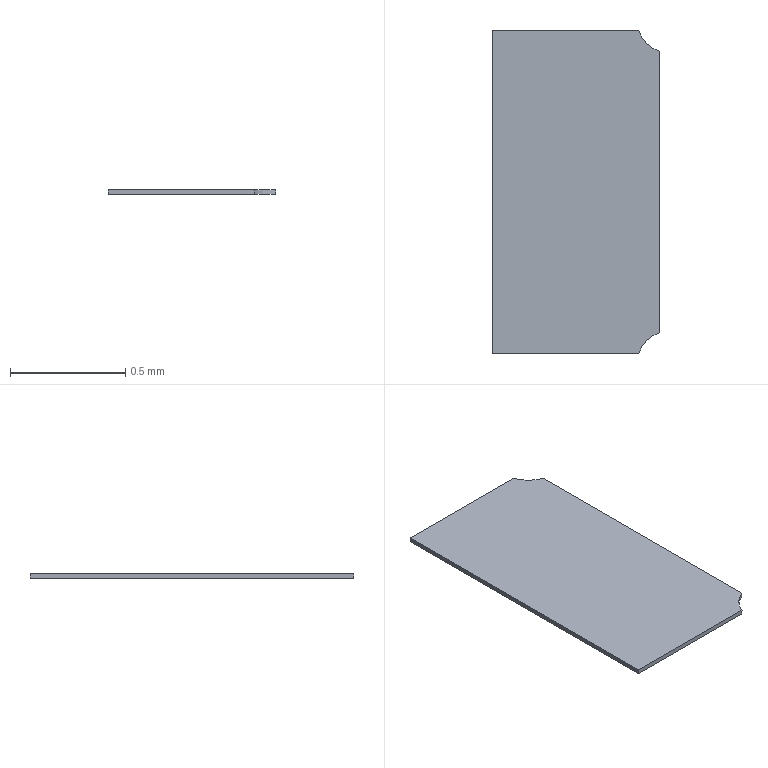Part | STEP file | RJ-USIO-V1_2-220411_229 | 1 solid | 8 faces | box 0.725 x 1.4 x 0.02 mm | volume 0.02008 mm3 | plane 6 | cylinder 2 | commonest cylinder face diameters 0.3 x2
STEP:
#1=CARTESIAN_POINT('',(0.,0.,0.));
#2=DIRECTION('',(0.,0.,1.));
#3=DIRECTION('',(1.,0.,0.));
#4=AXIS2_PLACEMENT_3D('',#1,#2,#3);
#5=CARTESIAN_POINT('',(41.209,55.9,0.000000031));
#6=VERTEX_POINT('',#5);
#7=CARTESIAN_POINT('',(41.3,55.808,0.000000027));
#8=VERTEX_POINT('',#7);
#9=CARTESIAN_POINT('',(41.35,55.95,0.000000033));
#10=DIRECTION('',(0.,-0.000000044,1.));
#11=DIRECTION('',(-0.9428,-0.3333,-0.000000015));
#12=AXIS2_PLACEMENT_3D('',#9,#10,#11);
#13=CIRCLE('',#12,0.15);
#14=CARTESIAN_POINT('',(41.35,55.95,0.000000033));
#15=DIRECTION('',(0.,0.000000044,-1.));
#16=DIRECTION('',(0.000000175,-1.,-0.000000044));
#17=AXIS2_PLACEMENT_3D('',#14,#15,#16);
#18=PLANE('',#17);
#19=CARTESIAN_POINT('',(0.05,0.1414));
#20=CARTESIAN_POINT('',(0.2949,0.05482));
#21=CARTESIAN_POINT('',(0.09747,-0.114));
#22=CARTESIAN_POINT('',(-0.1,-0.2828));
#23=CARTESIAN_POINT('',(-0.1475,-0.02741));
#24=CARTESIAN_POINT('',(-0.1949,0.228));
#25=CARTESIAN_POINT('',(0.05,0.1414));
#26=(BOUNDED_CURVE()B_SPLINE_CURVE(2,(#19,#20,#21,#22,#23,#24,#25),.UNSPECIFIED.,.T.,.F.)B_SPLINE_CURVE_WITH_KNOTS((1,2,2,2,2,1),(-2.094,0.,2.094,4.189,6.283,8.378),.UNSPECIFIED.)CURVE()GEOMETRIC_REPRESENTATION_ITEM()RATIONAL_B_SPLINE_CURVE((1.,0.5,1.,0.5,1.,0.5,1.))REPRESENTATION_ITEM(''));
#27=(GEOMETRIC_REPRESENTATION_CONTEXT(2)PARAMETRIC_REPRESENTATION_CONTEXT()REPRESENTATION_CONTEXT('',''));
#28=DEFINITIONAL_REPRESENTATION('',(#26),#27);
#29=PCURVE('',#18,#28);
#30=CARTESIAN_POINT('',(41.35,55.95,0.02));
#31=DIRECTION('',(0.,0.000000044,-1.));
#32=DIRECTION('',(0.000000175,-1.,-0.000000044));
#33=AXIS2_PLACEMENT_3D('',#30,#31,#32);
#34=CYLINDRICAL_SURFACE('',#33,0.15);
#35=CARTESIAN_POINT('',(1.231,0.02));
#36=DIRECTION('',(-1.,0.));
#37=VECTOR('',#36,1.);
#38=LINE('',#35,#37);
#39=(GEOMETRIC_REPRESENTATION_CONTEXT(2)PARAMETRIC_REPRESENTATION_CONTEXT()REPRESENTATION_CONTEXT('',''));
#40=DEFINITIONAL_REPRESENTATION('',(#38),#39);
#41=PCURVE('',#34,#40);
#42=SURFACE_CURVE('',#13,(#29,#41),.PCURVE_S1.);
#43=EDGE_CURVE('',#6,#8,#42,.T.);
#44=ORIENTED_EDGE('',*,*,#43,.F.);
#45=CARTESIAN_POINT('',(40.575,55.9,0.000000031));
#46=VERTEX_POINT('',#45);
#47=CARTESIAN_POINT('',(40.575,55.9,0.000000031));
#48=DIRECTION('',(1.,0.000000175,0.));
#49=VECTOR('',#48,1.);
#50=LINE('',#47,#49);
#51=CARTESIAN_POINT('',(0.05,0.775));
#52=DIRECTION('',(0.,-1.));
#53=VECTOR('',#52,1.);
#54=LINE('',#51,#53);
#55=(GEOMETRIC_REPRESENTATION_CONTEXT(2)PARAMETRIC_REPRESENTATION_CONTEXT()REPRESENTATION_CONTEXT('',''));
#56=DEFINITIONAL_REPRESENTATION('',(#54),#55);
#57=PCURVE('',#18,#56);
#58=CARTESIAN_POINT('',(41.209,55.9,0.02));
#59=DIRECTION('',(0.000000175,-1.,-0.000000044));
#60=DIRECTION('',(-1.,-0.000000175,0.));
#61=AXIS2_PLACEMENT_3D('',#58,#59,#60);
#62=PLANE('',#61);
#63=CARTESIAN_POINT('',(0.6336,0.02));
#64=DIRECTION('',(-1.,0.));
#65=VECTOR('',#64,1.);
#66=LINE('',#63,#65);
#67=(GEOMETRIC_REPRESENTATION_CONTEXT(2)PARAMETRIC_REPRESENTATION_CONTEXT()REPRESENTATION_CONTEXT('',''));
#68=DEFINITIONAL_REPRESENTATION('',(#66),#67);
#69=PCURVE('',#62,#68);
#70=SURFACE_CURVE('',#50,(#57,#69),.PCURVE_S1.);
#71=EDGE_CURVE('',#46,#6,#70,.T.);
#72=ORIENTED_EDGE('',*,*,#71,.F.);
#73=CARTESIAN_POINT('',(40.575,54.5,-0.000000031));
#74=VERTEX_POINT('',#73);
#75=CARTESIAN_POINT('',(40.575,54.5,-0.000000031));
#76=DIRECTION('',(-0.000000175,1.,0.000000044));
#77=VECTOR('',#76,1.);
#78=LINE('',#75,#77);
#79=CARTESIAN_POINT('',(1.45,0.775));
#80=DIRECTION('',(-1.,0.));
#81=VECTOR('',#80,1.);
#82=LINE('',#79,#81);
#83=(GEOMETRIC_REPRESENTATION_CONTEXT(2)PARAMETRIC_REPRESENTATION_CONTEXT()REPRESENTATION_CONTEXT('',''));
#84=DEFINITIONAL_REPRESENTATION('',(#82),#83);
#85=PCURVE('',#18,#84);
#86=CARTESIAN_POINT('',(40.575,55.9,0.02));
#87=DIRECTION('',(1.,0.000000175,0.));
#88=DIRECTION('',(0.000000175,-1.,-0.000000044));
#89=AXIS2_PLACEMENT_3D('',#86,#87,#88);
#90=PLANE('',#89);
#91=CARTESIAN_POINT('',(1.4,0.02));
#92=DIRECTION('',(-1.,0.));
#93=VECTOR('',#92,1.);
#94=LINE('',#91,#93);
#95=(GEOMETRIC_REPRESENTATION_CONTEXT(2)PARAMETRIC_REPRESENTATION_CONTEXT()REPRESENTATION_CONTEXT('',''));
#96=DEFINITIONAL_REPRESENTATION('',(#94),#95);
#97=PCURVE('',#90,#96);
#98=SURFACE_CURVE('',#78,(#85,#97),.PCURVE_S1.);
#99=EDGE_CURVE('',#74,#46,#98,.T.);
#100=ORIENTED_EDGE('',*,*,#99,.F.);
#101=CARTESIAN_POINT('',(41.209,54.5,-0.000000031));
#102=VERTEX_POINT('',#101);
#103=CARTESIAN_POINT('',(41.209,54.5,-0.000000031));
#104=DIRECTION('',(-1.,-0.000000175,0.));
#105=VECTOR('',#104,1.);
#106=LINE('',#103,#105);
#107=CARTESIAN_POINT('',(1.45,0.1414));
#108=DIRECTION('',(0.,1.));
#109=VECTOR('',#108,1.);
#110=LINE('',#107,#109);
#111=(GEOMETRIC_REPRESENTATION_CONTEXT(2)PARAMETRIC_REPRESENTATION_CONTEXT()REPRESENTATION_CONTEXT('',''));
#112=DEFINITIONAL_REPRESENTATION('',(#110),#111);
#113=PCURVE('',#18,#112);
#114=CARTESIAN_POINT('',(40.575,54.5,0.02));
#115=DIRECTION('',(-0.000000175,1.,0.000000044));
#116=DIRECTION('',(1.,0.000000175,0.));
#117=AXIS2_PLACEMENT_3D('',#114,#115,#116);
#118=PLANE('',#117);
#119=CARTESIAN_POINT('',(0.6336,0.02));
#120=DIRECTION('',(-1.,0.));
#121=VECTOR('',#120,1.);
#122=LINE('',#119,#121);
#123=(GEOMETRIC_REPRESENTATION_CONTEXT(2)PARAMETRIC_REPRESENTATION_CONTEXT()REPRESENTATION_CONTEXT('',''));
#124=DEFINITIONAL_REPRESENTATION('',(#122),#123);
#125=PCURVE('',#118,#124);
#126=SURFACE_CURVE('',#106,(#113,#125),.PCURVE_S1.);
#127=EDGE_CURVE('',#102,#74,#126,.T.);
#128=ORIENTED_EDGE('',*,*,#127,.F.);
#129=CARTESIAN_POINT('',(41.3,54.591,-0.000000027));
#130=VERTEX_POINT('',#129);
#131=CARTESIAN_POINT('',(41.35,54.45,-0.000000033));
#132=DIRECTION('',(0.,-0.000000044,1.));
#133=DIRECTION('',(-0.3333,0.9428,0.000000041));
#134=AXIS2_PLACEMENT_3D('',#131,#132,#133);
#135=CIRCLE('',#134,0.15);
#136=CARTESIAN_POINT('',(1.359,0.05));
#137=CARTESIAN_POINT('',(1.445,0.2949));
#138=CARTESIAN_POINT('',(1.614,0.09747));
#139=CARTESIAN_POINT('',(1.783,-0.1));
#140=CARTESIAN_POINT('',(1.527,-0.1475));
#141=CARTESIAN_POINT('',(1.272,-0.1949));
#142=CARTESIAN_POINT('',(1.359,0.05));
#143=(BOUNDED_CURVE()B_SPLINE_CURVE(2,(#136,#137,#138,#139,#140,#141,#142),.UNSPECIFIED.,.T.,.F.)B_SPLINE_CURVE_WITH_KNOTS((1,2,2,2,2,1),(-2.094,0.,2.094,4.189,6.283,8.378),.UNSPECIFIED.)CURVE()GEOMETRIC_REPRESENTATION_ITEM()RATIONAL_B_SPLINE_CURVE((1.,0.5,1.,0.5,1.,0.5,1.))REPRESENTATION_ITEM(''));
#144=(GEOMETRIC_REPRESENTATION_CONTEXT(2)PARAMETRIC_REPRESENTATION_CONTEXT()REPRESENTATION_CONTEXT('',''));
#145=DEFINITIONAL_REPRESENTATION('',(#143),#144);
#146=PCURVE('',#18,#145);
#147=CARTESIAN_POINT('',(41.35,54.45,0.02));
#148=DIRECTION('',(0.,0.000000044,-1.));
#149=DIRECTION('',(0.000000175,-1.,-0.000000044));
#150=AXIS2_PLACEMENT_3D('',#147,#148,#149);
#151=CYLINDRICAL_SURFACE('',#150,0.15);
#152=CARTESIAN_POINT('',(2.802,0.02));
#153=DIRECTION('',(-1.,0.));
#154=VECTOR('',#153,1.);
#155=LINE('',#152,#154);
#156=(GEOMETRIC_REPRESENTATION_CONTEXT(2)PARAMETRIC_REPRESENTATION_CONTEXT()REPRESENTATION_CONTEXT('',''));
#157=DEFINITIONAL_REPRESENTATION('',(#155),#156);
#158=PCURVE('',#151,#157);
#159=SURFACE_CURVE('',#135,(#146,#158),.PCURVE_S1.);
#160=EDGE_CURVE('',#130,#102,#159,.T.);
#161=ORIENTED_EDGE('',*,*,#160,.F.);
#162=CARTESIAN_POINT('',(41.3,55.808,0.000000027));
#163=DIRECTION('',(0.000000175,-1.,-0.000000044));
#164=VECTOR('',#163,1.);
#165=LINE('',#162,#164);
#166=CARTESIAN_POINT('',(0.1414,0.05));
#167=DIRECTION('',(1.,0.));
#168=VECTOR('',#167,1.);
#169=LINE('',#166,#168);
#170=(GEOMETRIC_REPRESENTATION_CONTEXT(2)PARAMETRIC_REPRESENTATION_CONTEXT()REPRESENTATION_CONTEXT('',''));
#171=DEFINITIONAL_REPRESENTATION('',(#169),#170);
#172=PCURVE('',#18,#171);
#173=CARTESIAN_POINT('',(41.3,55.808,0.02));
#174=DIRECTION('',(-1.,-0.000000175,0.));
#175=DIRECTION('',(-0.000000175,1.,0.000000044));
#176=AXIS2_PLACEMENT_3D('',#173,#174,#175);
#177=PLANE('',#176);
#178=CARTESIAN_POINT('',(0.,0.02));
#179=DIRECTION('',(-1.,0.));
#180=VECTOR('',#179,1.);
#181=LINE('',#178,#180);
#182=(GEOMETRIC_REPRESENTATION_CONTEXT(2)PARAMETRIC_REPRESENTATION_CONTEXT()REPRESENTATION_CONTEXT('',''));
#183=DEFINITIONAL_REPRESENTATION('',(#181),#182);
#184=PCURVE('',#177,#183);
#185=SURFACE_CURVE('',#165,(#172,#184),.PCURVE_S1.);
#186=EDGE_CURVE('',#8,#130,#185,.T.);
#187=ORIENTED_EDGE('',*,*,#186,.F.);
#188=EDGE_LOOP('',(#44,#72,#100,#128,#161,#187));
#189=FACE_BOUND('',#188,.F.);
#190=ADVANCED_FACE('',(#189),#18,.T.);
#191=ORIENTED_EDGE('',*,*,#43,.T.);
#192=CARTESIAN_POINT('',(41.3,55.808,0.02));
#193=VERTEX_POINT('',#192);
#194=CARTESIAN_POINT('',(41.3,55.808,0.02));
#195=DIRECTION('',(0.,0.000000044,-1.));
#196=VECTOR('',#195,1.);
#197=LINE('',#194,#196);
#198=CARTESIAN_POINT('',(0.3398,0.));
#199=DIRECTION('',(0.,1.));
#200=VECTOR('',#199,1.);
#201=LINE('',#198,#200);
#202=(GEOMETRIC_REPRESENTATION_CONTEXT(2)PARAMETRIC_REPRESENTATION_CONTEXT()REPRESENTATION_CONTEXT('',''));
#203=DEFINITIONAL_REPRESENTATION('',(#201),#202);
#204=PCURVE('',#34,#203);
#205=CARTESIAN_POINT('',(0.,0.));
#206=DIRECTION('',(0.,1.));
#207=VECTOR('',#206,1.);
#208=LINE('',#205,#207);
#209=(GEOMETRIC_REPRESENTATION_CONTEXT(2)PARAMETRIC_REPRESENTATION_CONTEXT()REPRESENTATION_CONTEXT('',''));
#210=DEFINITIONAL_REPRESENTATION('',(#208),#209);
#211=PCURVE('',#177,#210);
#212=SURFACE_CURVE('',#197,(#204,#211),.PCURVE_S1.);
#213=EDGE_CURVE('',#193,#8,#212,.T.);
#214=ORIENTED_EDGE('',*,*,#213,.F.);
#215=CARTESIAN_POINT('',(41.209,55.9,0.02));
#216=VERTEX_POINT('',#215);
#217=CARTESIAN_POINT('',(41.35,55.95,0.02));
#218=DIRECTION('',(0.,0.000000044,-1.));
#219=DIRECTION('',(-0.3333,-0.9428,-0.000000041));
#220=AXIS2_PLACEMENT_3D('',#217,#218,#219);
#221=CIRCLE('',#220,0.15);
#222=CARTESIAN_POINT('',(0.3398,0.));
#223=DIRECTION('',(1.,0.));
#224=VECTOR('',#223,1.);
#225=LINE('',#222,#224);
#226=(GEOMETRIC_REPRESENTATION_CONTEXT(2)PARAMETRIC_REPRESENTATION_CONTEXT()REPRESENTATION_CONTEXT('',''));
#227=DEFINITIONAL_REPRESENTATION('',(#225),#226);
#228=PCURVE('',#34,#227);
#229=CARTESIAN_POINT('',(41.35,55.95,0.02));
#230=DIRECTION('',(0.,0.000000044,-1.));
#231=DIRECTION('',(0.000000175,-1.,-0.000000044));
#232=AXIS2_PLACEMENT_3D('',#229,#230,#231);
#233=PLANE('',#232);
#234=CARTESIAN_POINT('',(0.,0.));
#235=DIRECTION('',(0.9428,0.3333));
#236=AXIS2_PLACEMENT_2D('',#234,#235);
#237=CIRCLE('',#236,0.15);
#238=(GEOMETRIC_REPRESENTATION_CONTEXT(2)PARAMETRIC_REPRESENTATION_CONTEXT()REPRESENTATION_CONTEXT('',''));
#239=DEFINITIONAL_REPRESENTATION('',(#237),#238);
#240=PCURVE('',#233,#239);
#241=SURFACE_CURVE('',#221,(#228,#240),.PCURVE_S1.);
#242=EDGE_CURVE('',#193,#216,#241,.T.);
#243=ORIENTED_EDGE('',*,*,#242,.T.);
#244=CARTESIAN_POINT('',(41.209,55.9,0.000000031));
#245=DIRECTION('',(0.,-0.000000044,1.));
#246=VECTOR('',#245,1.);
#247=LINE('',#244,#246);
#248=CARTESIAN_POINT('',(1.231,0.02));
#249=DIRECTION('',(0.,-1.));
#250=VECTOR('',#249,1.);
#251=LINE('',#248,#250);
#252=(GEOMETRIC_REPRESENTATION_CONTEXT(2)PARAMETRIC_REPRESENTATION_CONTEXT()REPRESENTATION_CONTEXT('',''));
#253=DEFINITIONAL_REPRESENTATION('',(#251),#252);
#254=PCURVE('',#34,#253);
#255=CARTESIAN_POINT('',(0.,0.02));
#256=DIRECTION('',(0.,-1.));
#257=VECTOR('',#256,1.);
#258=LINE('',#255,#257);
#259=(GEOMETRIC_REPRESENTATION_CONTEXT(2)PARAMETRIC_REPRESENTATION_CONTEXT()REPRESENTATION_CONTEXT('',''));
#260=DEFINITIONAL_REPRESENTATION('',(#258),#259);
#261=PCURVE('',#62,#260);
#262=SURFACE_CURVE('',#247,(#254,#261),.PCURVE_S1.);
#263=EDGE_CURVE('',#6,#216,#262,.T.);
#264=ORIENTED_EDGE('',*,*,#263,.F.);
#265=EDGE_LOOP('',(#191,#214,#243,#264));
#266=FACE_BOUND('',#265,.F.);
#267=ADVANCED_FACE('',(#266),#34,.F.);
#268=ORIENTED_EDGE('',*,*,#186,.T.);
#269=CARTESIAN_POINT('',(41.3,54.591,0.02));
#270=VERTEX_POINT('',#269);
#271=CARTESIAN_POINT('',(41.3,54.591,-0.000000027));
#272=DIRECTION('',(0.,-0.000000044,1.));
#273=VECTOR('',#272,1.);
#274=LINE('',#271,#273);
#275=CARTESIAN_POINT('',(-1.217,0.02));
#276=DIRECTION('',(0.,-1.));
#277=VECTOR('',#276,1.);
#278=LINE('',#275,#277);
#279=(GEOMETRIC_REPRESENTATION_CONTEXT(2)PARAMETRIC_REPRESENTATION_CONTEXT()REPRESENTATION_CONTEXT('',''));
#280=DEFINITIONAL_REPRESENTATION('',(#278),#279);
#281=PCURVE('',#177,#280);
#282=CARTESIAN_POINT('',(2.802,0.02));
#283=DIRECTION('',(0.,-1.));
#284=VECTOR('',#283,1.);
#285=LINE('',#282,#284);
#286=(GEOMETRIC_REPRESENTATION_CONTEXT(2)PARAMETRIC_REPRESENTATION_CONTEXT()REPRESENTATION_CONTEXT('',''));
#287=DEFINITIONAL_REPRESENTATION('',(#285),#286);
#288=PCURVE('',#151,#287);
#289=SURFACE_CURVE('',#274,(#281,#288),.PCURVE_S1.);
#290=EDGE_CURVE('',#130,#270,#289,.T.);
#291=ORIENTED_EDGE('',*,*,#290,.T.);
#292=CARTESIAN_POINT('',(41.3,55.808,0.02));
#293=DIRECTION('',(0.000000175,-1.,-0.000000044));
#294=VECTOR('',#293,1.);
#295=LINE('',#292,#294);
#296=CARTESIAN_POINT('',(0.,0.));
#297=DIRECTION('',(-1.,0.));
#298=VECTOR('',#297,1.);
#299=LINE('',#296,#298);
#300=(GEOMETRIC_REPRESENTATION_CONTEXT(2)PARAMETRIC_REPRESENTATION_CONTEXT()REPRESENTATION_CONTEXT('',''));
#301=DEFINITIONAL_REPRESENTATION('',(#299),#300);
#302=PCURVE('',#177,#301);
#303=CARTESIAN_POINT('',(0.1414,0.05));
#304=DIRECTION('',(1.,0.));
#305=VECTOR('',#304,1.);
#306=LINE('',#303,#305);
#307=(GEOMETRIC_REPRESENTATION_CONTEXT(2)PARAMETRIC_REPRESENTATION_CONTEXT()REPRESENTATION_CONTEXT('',''));
#308=DEFINITIONAL_REPRESENTATION('',(#306),#307);
#309=PCURVE('',#233,#308);
#310=SURFACE_CURVE('',#295,(#302,#309),.PCURVE_S1.);
#311=EDGE_CURVE('',#193,#270,#310,.T.);
#312=ORIENTED_EDGE('',*,*,#311,.F.);
#313=ORIENTED_EDGE('',*,*,#213,.T.);
#314=EDGE_LOOP('',(#268,#291,#312,#313));
#315=FACE_BOUND('',#314,.F.);
#316=ADVANCED_FACE('',(#315),#177,.F.);
#317=ORIENTED_EDGE('',*,*,#160,.T.);
#318=CARTESIAN_POINT('',(41.209,54.5,0.02));
#319=VERTEX_POINT('',#318);
#320=CARTESIAN_POINT('',(41.209,54.5,0.02));
#321=DIRECTION('',(0.,0.000000044,-1.));
#322=VECTOR('',#321,1.);
#323=LINE('',#320,#322);
#324=CARTESIAN_POINT('',(1.911,0.));
#325=DIRECTION('',(0.,1.));
#326=VECTOR('',#325,1.);
#327=LINE('',#324,#326);
#328=(GEOMETRIC_REPRESENTATION_CONTEXT(2)PARAMETRIC_REPRESENTATION_CONTEXT()REPRESENTATION_CONTEXT('',''));
#329=DEFINITIONAL_REPRESENTATION('',(#327),#328);
#330=PCURVE('',#151,#329);
#331=CARTESIAN_POINT('',(0.6336,0.));
#332=DIRECTION('',(0.,1.));
#333=VECTOR('',#332,1.);
#334=LINE('',#331,#333);
#335=(GEOMETRIC_REPRESENTATION_CONTEXT(2)PARAMETRIC_REPRESENTATION_CONTEXT()REPRESENTATION_CONTEXT('',''));
#336=DEFINITIONAL_REPRESENTATION('',(#334),#335);
#337=PCURVE('',#118,#336);
#338=SURFACE_CURVE('',#323,(#330,#337),.PCURVE_S1.);
#339=EDGE_CURVE('',#319,#102,#338,.T.);
#340=ORIENTED_EDGE('',*,*,#339,.F.);
#341=CARTESIAN_POINT('',(41.35,54.45,0.02));
#342=DIRECTION('',(0.,0.000000044,-1.));
#343=DIRECTION('',(-0.9428,0.3333,0.000000015));
#344=AXIS2_PLACEMENT_3D('',#341,#342,#343);
#345=CIRCLE('',#344,0.15);
#346=CARTESIAN_POINT('',(1.911,0.));
#347=DIRECTION('',(1.,0.));
#348=VECTOR('',#347,1.);
#349=LINE('',#346,#348);
#350=(GEOMETRIC_REPRESENTATION_CONTEXT(2)PARAMETRIC_REPRESENTATION_CONTEXT()REPRESENTATION_CONTEXT('',''));
#351=DEFINITIONAL_REPRESENTATION('',(#349),#350);
#352=PCURVE('',#151,#351);
#353=CARTESIAN_POINT('',(1.5,0.));
#354=DIRECTION('',(-0.3333,0.9428));
#355=AXIS2_PLACEMENT_2D('',#353,#354);
#356=CIRCLE('',#355,0.15);
#357=(GEOMETRIC_REPRESENTATION_CONTEXT(2)PARAMETRIC_REPRESENTATION_CONTEXT()REPRESENTATION_CONTEXT('',''));
#358=DEFINITIONAL_REPRESENTATION('',(#356),#357);
#359=PCURVE('',#233,#358);
#360=SURFACE_CURVE('',#345,(#352,#359),.PCURVE_S1.);
#361=EDGE_CURVE('',#319,#270,#360,.T.);
#362=ORIENTED_EDGE('',*,*,#361,.T.);
#363=ORIENTED_EDGE('',*,*,#290,.F.);
#364=EDGE_LOOP('',(#317,#340,#362,#363));
#365=FACE_BOUND('',#364,.F.);
#366=ADVANCED_FACE('',(#365),#151,.F.);
#367=ORIENTED_EDGE('',*,*,#127,.T.);
#368=CARTESIAN_POINT('',(40.575,54.5,0.02));
#369=VERTEX_POINT('',#368);
#370=CARTESIAN_POINT('',(40.575,54.5,-0.000000031));
#371=DIRECTION('',(0.,-0.000000044,1.));
#372=VECTOR('',#371,1.);
#373=LINE('',#370,#372);
#374=CARTESIAN_POINT('',(0.,0.02));
#375=DIRECTION('',(0.,-1.));
#376=VECTOR('',#375,1.);
#377=LINE('',#374,#376);
#378=(GEOMETRIC_REPRESENTATION_CONTEXT(2)PARAMETRIC_REPRESENTATION_CONTEXT()REPRESENTATION_CONTEXT('',''));
#379=DEFINITIONAL_REPRESENTATION('',(#377),#378);
#380=PCURVE('',#118,#379);
#381=CARTESIAN_POINT('',(1.4,0.02));
#382=DIRECTION('',(0.,-1.));
#383=VECTOR('',#382,1.);
#384=LINE('',#381,#383);
#385=(GEOMETRIC_REPRESENTATION_CONTEXT(2)PARAMETRIC_REPRESENTATION_CONTEXT()REPRESENTATION_CONTEXT('',''));
#386=DEFINITIONAL_REPRESENTATION('',(#384),#385);
#387=PCURVE('',#90,#386);
#388=SURFACE_CURVE('',#373,(#380,#387),.PCURVE_S1.);
#389=EDGE_CURVE('',#74,#369,#388,.T.);
#390=ORIENTED_EDGE('',*,*,#389,.T.);
#391=CARTESIAN_POINT('',(41.209,54.5,0.02));
#392=DIRECTION('',(-1.,-0.000000175,0.));
#393=VECTOR('',#392,1.);
#394=LINE('',#391,#393);
#395=CARTESIAN_POINT('',(0.6336,0.));
#396=DIRECTION('',(-1.,0.));
#397=VECTOR('',#396,1.);
#398=LINE('',#395,#397);
#399=(GEOMETRIC_REPRESENTATION_CONTEXT(2)PARAMETRIC_REPRESENTATION_CONTEXT()REPRESENTATION_CONTEXT('',''));
#400=DEFINITIONAL_REPRESENTATION('',(#398),#399);
#401=PCURVE('',#118,#400);
#402=CARTESIAN_POINT('',(1.45,0.1414));
#403=DIRECTION('',(0.,1.));
#404=VECTOR('',#403,1.);
#405=LINE('',#402,#404);
#406=(GEOMETRIC_REPRESENTATION_CONTEXT(2)PARAMETRIC_REPRESENTATION_CONTEXT()REPRESENTATION_CONTEXT('',''));
#407=DEFINITIONAL_REPRESENTATION('',(#405),#406);
#408=PCURVE('',#233,#407);
#409=SURFACE_CURVE('',#394,(#401,#408),.PCURVE_S1.);
#410=EDGE_CURVE('',#319,#369,#409,.T.);
#411=ORIENTED_EDGE('',*,*,#410,.F.);
#412=ORIENTED_EDGE('',*,*,#339,.T.);
#413=EDGE_LOOP('',(#367,#390,#411,#412));
#414=FACE_BOUND('',#413,.F.);
#415=ADVANCED_FACE('',(#414),#118,.F.);
#416=ORIENTED_EDGE('',*,*,#99,.T.);
#417=CARTESIAN_POINT('',(40.575,55.9,0.02));
#418=VERTEX_POINT('',#417);
#419=CARTESIAN_POINT('',(40.575,55.9,0.000000031));
#420=DIRECTION('',(0.,-0.000000044,1.));
#421=VECTOR('',#420,1.);
#422=LINE('',#419,#421);
#423=CARTESIAN_POINT('',(0.,0.02));
#424=DIRECTION('',(0.,-1.));
#425=VECTOR('',#424,1.);
#426=LINE('',#423,#425);
#427=(GEOMETRIC_REPRESENTATION_CONTEXT(2)PARAMETRIC_REPRESENTATION_CONTEXT()REPRESENTATION_CONTEXT('',''));
#428=DEFINITIONAL_REPRESENTATION('',(#426),#427);
#429=PCURVE('',#90,#428);
#430=CARTESIAN_POINT('',(0.6336,0.02));
#431=DIRECTION('',(0.,-1.));
#432=VECTOR('',#431,1.);
#433=LINE('',#430,#432);
#434=(GEOMETRIC_REPRESENTATION_CONTEXT(2)PARAMETRIC_REPRESENTATION_CONTEXT()REPRESENTATION_CONTEXT('',''));
#435=DEFINITIONAL_REPRESENTATION('',(#433),#434);
#436=PCURVE('',#62,#435);
#437=SURFACE_CURVE('',#422,(#429,#436),.PCURVE_S1.);
#438=EDGE_CURVE('',#46,#418,#437,.T.);
#439=ORIENTED_EDGE('',*,*,#438,.T.);
#440=CARTESIAN_POINT('',(40.575,54.5,0.02));
#441=DIRECTION('',(-0.000000175,1.,0.000000044));
#442=VECTOR('',#441,1.);
#443=LINE('',#440,#442);
#444=CARTESIAN_POINT('',(1.4,0.));
#445=DIRECTION('',(-1.,0.));
#446=VECTOR('',#445,1.);
#447=LINE('',#444,#446);
#448=(GEOMETRIC_REPRESENTATION_CONTEXT(2)PARAMETRIC_REPRESENTATION_CONTEXT()REPRESENTATION_CONTEXT('',''));
#449=DEFINITIONAL_REPRESENTATION('',(#447),#448);
#450=PCURVE('',#90,#449);
#451=CARTESIAN_POINT('',(1.45,0.775));
#452=DIRECTION('',(-1.,0.));
#453=VECTOR('',#452,1.);
#454=LINE('',#451,#453);
#455=(GEOMETRIC_REPRESENTATION_CONTEXT(2)PARAMETRIC_REPRESENTATION_CONTEXT()REPRESENTATION_CONTEXT('',''));
#456=DEFINITIONAL_REPRESENTATION('',(#454),#455);
#457=PCURVE('',#233,#456);
#458=SURFACE_CURVE('',#443,(#450,#457),.PCURVE_S1.);
#459=EDGE_CURVE('',#369,#418,#458,.T.);
#460=ORIENTED_EDGE('',*,*,#459,.F.);
#461=ORIENTED_EDGE('',*,*,#389,.F.);
#462=EDGE_LOOP('',(#416,#439,#460,#461));
#463=FACE_BOUND('',#462,.F.);
#464=ADVANCED_FACE('',(#463),#90,.F.);
#465=ORIENTED_EDGE('',*,*,#71,.T.);
#466=ORIENTED_EDGE('',*,*,#263,.T.);
#467=CARTESIAN_POINT('',(40.575,55.9,0.02));
#468=DIRECTION('',(1.,0.000000175,0.));
#469=VECTOR('',#468,1.);
#470=LINE('',#467,#469);
#471=CARTESIAN_POINT('',(0.6336,0.));
#472=DIRECTION('',(-1.,0.));
#473=VECTOR('',#472,1.);
#474=LINE('',#471,#473);
#475=(GEOMETRIC_REPRESENTATION_CONTEXT(2)PARAMETRIC_REPRESENTATION_CONTEXT()REPRESENTATION_CONTEXT('',''));
#476=DEFINITIONAL_REPRESENTATION('',(#474),#475);
#477=PCURVE('',#62,#476);
#478=CARTESIAN_POINT('',(0.05,0.775));
#479=DIRECTION('',(0.,-1.));
#480=VECTOR('',#479,1.);
#481=LINE('',#478,#480);
#482=(GEOMETRIC_REPRESENTATION_CONTEXT(2)PARAMETRIC_REPRESENTATION_CONTEXT()REPRESENTATION_CONTEXT('',''));
#483=DEFINITIONAL_REPRESENTATION('',(#481),#482);
#484=PCURVE('',#233,#483);
#485=SURFACE_CURVE('',#470,(#477,#484),.PCURVE_S1.);
#486=EDGE_CURVE('',#418,#216,#485,.T.);
#487=ORIENTED_EDGE('',*,*,#486,.F.);
#488=ORIENTED_EDGE('',*,*,#438,.F.);
#489=EDGE_LOOP('',(#465,#466,#487,#488));
#490=FACE_BOUND('',#489,.F.);
#491=ADVANCED_FACE('',(#490),#62,.F.);
#492=ORIENTED_EDGE('',*,*,#242,.F.);
#493=ORIENTED_EDGE('',*,*,#311,.T.);
#494=ORIENTED_EDGE('',*,*,#361,.F.);
#495=ORIENTED_EDGE('',*,*,#410,.T.);
#496=ORIENTED_EDGE('',*,*,#459,.T.);
#497=ORIENTED_EDGE('',*,*,#486,.T.);
#498=EDGE_LOOP('',(#492,#493,#494,#495,#496,#497));
#499=FACE_BOUND('',#498,.F.);
#500=ADVANCED_FACE('',(#499),#233,.F.);
#501=CLOSED_SHELL('',(#190,#267,#316,#366,#415,#464,#491,#500));
#502=MANIFOLD_SOLID_BREP('',#501);
#503=(LENGTH_UNIT()NAMED_UNIT(*)SI_UNIT(.MILLI.,.METRE.));
#504=UNCERTAINTY_MEASURE_WITH_UNIT(LENGTH_MEASURE(0.0000001),#503,'','');
#505=(NAMED_UNIT(*)PLANE_ANGLE_UNIT()SI_UNIT($,.RADIAN.));
#506=(NAMED_UNIT(*)SI_UNIT($,.STERADIAN.)SOLID_ANGLE_UNIT());
#507=(GEOMETRIC_REPRESENTATION_CONTEXT(3)GLOBAL_UNCERTAINTY_ASSIGNED_CONTEXT((#504))GLOBAL_UNIT_ASSIGNED_CONTEXT((#503,#505,#506))REPRESENTATION_CONTEXT('',''));
#508=ADVANCED_BREP_SHAPE_REPRESENTATION('',(#4,#502),#507);